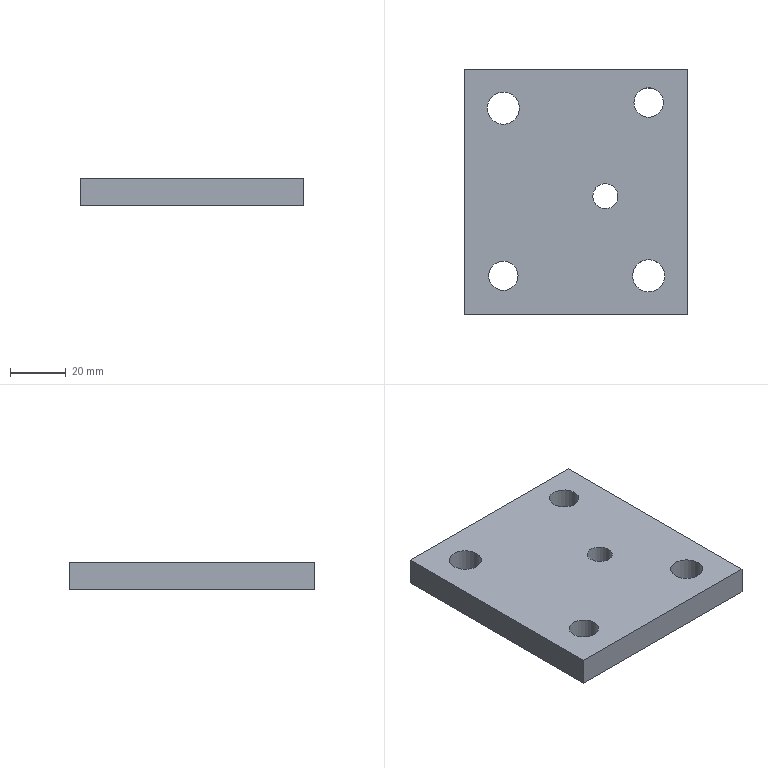Part | NX | features 6 2 | 1 solid | 11 faces | box 80 x 88 x 10 mm | volume 65955 mm3 | plane 6 | cylinder 5 | commonest cylinder face diameters 10.5 x2 11.5 x2 9 x1
STEP:
#1=CARTESIAN_POINT('',(3340.247,122.828,101.));
#2=VERTEX_POINT('',#1);
#3=CARTESIAN_POINT('',(3340.247,34.828,101.));
#4=VERTEX_POINT('',#3);
#5=CARTESIAN_POINT('',(3340.247,77.328,101.));
#6=DIRECTION('',(0.,-1.,0.));
#7=VECTOR('',#6,1000.);
#8=LINE('',#5,#7);
#9=EDGE_CURVE('',#2,#4,#8,.T.);
#10=ORIENTED_EDGE('',*,*,#9,.T.);
#11=CARTESIAN_POINT('',(3340.247,34.828,91.));
#12=VERTEX_POINT('',#11);
#13=CARTESIAN_POINT('',(3340.247,34.828,81.));
#14=DIRECTION('',(0.,0.,1.));
#15=VECTOR('',#14,1000.);
#16=LINE('',#13,#15);
#17=EDGE_CURVE('',#12,#4,#16,.T.);
#18=ORIENTED_EDGE('',*,*,#17,.F.);
#19=CARTESIAN_POINT('',(3340.247,122.828,91.));
#20=VERTEX_POINT('',#19);
#21=CARTESIAN_POINT('',(3340.247,77.328,91.));
#22=DIRECTION('',(0.,-1.,0.));
#23=VECTOR('',#22,1000.);
#24=LINE('',#21,#23);
#25=EDGE_CURVE('',#20,#12,#24,.T.);
#26=ORIENTED_EDGE('',*,*,#25,.F.);
#27=CARTESIAN_POINT('',(3340.247,122.828,81.));
#28=DIRECTION('',(0.,0.,-1.));
#29=VECTOR('',#28,1000.);
#30=LINE('',#27,#29);
#31=EDGE_CURVE('',#2,#20,#30,.T.);
#32=ORIENTED_EDGE('',*,*,#31,.F.);
#33=EDGE_LOOP('',(#10,#18,#26,#32));
#34=FACE_BOUND('',#33,.T.);
#35=CARTESIAN_POINT('',(3340.247,77.328,81.));
#36=DIRECTION('',(-1.,0.,0.));
#37=DIRECTION('',(0.,-1.,0.));
#38=AXIS2_PLACEMENT_3D('',#35,#36,#37);
#39=PLANE('',#38);
#40=ADVANCED_FACE('',(#34),#39,.F.);
#41=CARTESIAN_POINT('',(3260.247,122.828,101.));
#42=VERTEX_POINT('',#41);
#43=CARTESIAN_POINT('',(3290.247,122.828,101.));
#44=DIRECTION('',(1.,0.,0.));
#45=VECTOR('',#44,1000.);
#46=LINE('',#43,#45);
#47=EDGE_CURVE('',#42,#2,#46,.T.);
#48=ORIENTED_EDGE('',*,*,#47,.T.);
#49=ORIENTED_EDGE('',*,*,#31,.T.);
#50=CARTESIAN_POINT('',(3260.247,122.828,91.));
#51=VERTEX_POINT('',#50);
#52=CARTESIAN_POINT('',(3290.247,122.828,91.));
#53=DIRECTION('',(1.,0.,0.));
#54=VECTOR('',#53,1000.);
#55=LINE('',#52,#54);
#56=EDGE_CURVE('',#51,#20,#55,.T.);
#57=ORIENTED_EDGE('',*,*,#56,.F.);
#58=CARTESIAN_POINT('',(3260.247,122.828,81.));
#59=DIRECTION('',(0.,0.,-1.));
#60=VECTOR('',#59,1000.);
#61=LINE('',#58,#60);
#62=EDGE_CURVE('',#42,#51,#61,.T.);
#63=ORIENTED_EDGE('',*,*,#62,.F.);
#64=EDGE_LOOP('',(#48,#49,#57,#63));
#65=FACE_BOUND('',#64,.T.);
#66=CARTESIAN_POINT('',(3290.247,122.828,81.));
#67=DIRECTION('',(0.,-1.,0.));
#68=DIRECTION('',(1.,0.,0.));
#69=AXIS2_PLACEMENT_3D('',#66,#67,#68);
#70=PLANE('',#69);
#71=ADVANCED_FACE('',(#65),#70,.F.);
#72=CARTESIAN_POINT('',(3260.247,34.828,101.));
#73=VERTEX_POINT('',#72);
#74=CARTESIAN_POINT('',(3260.247,77.328,101.));
#75=DIRECTION('',(0.,1.,0.));
#76=VECTOR('',#75,1000.);
#77=LINE('',#74,#76);
#78=EDGE_CURVE('',#73,#42,#77,.T.);
#79=ORIENTED_EDGE('',*,*,#78,.T.);
#80=ORIENTED_EDGE('',*,*,#62,.T.);
#81=CARTESIAN_POINT('',(3260.247,34.828,91.));
#82=VERTEX_POINT('',#81);
#83=CARTESIAN_POINT('',(3260.247,77.328,91.));
#84=DIRECTION('',(0.,1.,0.));
#85=VECTOR('',#84,1000.);
#86=LINE('',#83,#85);
#87=EDGE_CURVE('',#82,#51,#86,.T.);
#88=ORIENTED_EDGE('',*,*,#87,.F.);
#89=CARTESIAN_POINT('',(3260.247,34.828,81.));
#90=DIRECTION('',(0.,0.,-1.));
#91=VECTOR('',#90,1000.);
#92=LINE('',#89,#91);
#93=EDGE_CURVE('',#73,#82,#92,.T.);
#94=ORIENTED_EDGE('',*,*,#93,.F.);
#95=EDGE_LOOP('',(#79,#80,#88,#94));
#96=FACE_BOUND('',#95,.T.);
#97=CARTESIAN_POINT('',(3260.247,77.328,81.));
#98=DIRECTION('',(1.,0.,0.));
#99=DIRECTION('',(0.,1.,0.));
#100=AXIS2_PLACEMENT_3D('',#97,#98,#99);
#101=PLANE('',#100);
#102=ADVANCED_FACE('',(#96),#101,.F.);
#103=CARTESIAN_POINT('',(3279.497,48.828,91.));
#104=VERTEX_POINT('',#103);
#105=CARTESIAN_POINT('',(3274.247,48.828,91.));
#106=DIRECTION('',(0.,0.,-1.));
#107=DIRECTION('',(1.,0.,0.));
#108=AXIS2_PLACEMENT_3D('',#105,#106,#107);
#109=CIRCLE('',#108,5.25);
#110=EDGE_CURVE('',#104,#104,#109,.T.);
#111=ORIENTED_EDGE('',*,*,#110,.T.);
#112=EDGE_LOOP('',(#111));
#113=FACE_BOUND('',#112,.T.);
#114=CARTESIAN_POINT('',(3268.997,48.828,101.));
#115=VERTEX_POINT('',#114);
#116=CARTESIAN_POINT('',(3274.247,48.828,101.));
#117=DIRECTION('',(0.,0.,1.));
#118=DIRECTION('',(-1.,0.,0.));
#119=AXIS2_PLACEMENT_3D('',#116,#117,#118);
#120=CIRCLE('',#119,5.25);
#121=EDGE_CURVE('',#115,#115,#120,.T.);
#122=ORIENTED_EDGE('',*,*,#121,.T.);
#123=EDGE_LOOP('',(#122));
#124=FACE_BOUND('',#123,.T.);
#125=CARTESIAN_POINT('',(3274.247,48.828,81.));
#126=DIRECTION('',(0.,0.,1.));
#127=DIRECTION('',(0.,-1.,0.));
#128=AXIS2_PLACEMENT_3D('',#125,#126,#127);
#129=CYLINDRICAL_SURFACE('',#128,5.25);
#130=ADVANCED_FACE('',(#113,#124),#129,.F.);
#131=CARTESIAN_POINT('',(3331.997,48.828,91.));
#132=VERTEX_POINT('',#131);
#133=CARTESIAN_POINT('',(3326.247,48.828,91.));
#134=DIRECTION('',(0.,0.,1.));
#135=DIRECTION('',(1.,0.,0.));
#136=AXIS2_PLACEMENT_3D('',#133,#134,#135);
#137=CIRCLE('',#136,5.75);
#138=EDGE_CURVE('',#132,#132,#137,.T.);
#139=ORIENTED_EDGE('',*,*,#138,.F.);
#140=EDGE_LOOP('',(#139));
#141=FACE_BOUND('',#140,.T.);
#142=CARTESIAN_POINT('',(3320.497,48.828,101.));
#143=VERTEX_POINT('',#142);
#144=CARTESIAN_POINT('',(3326.247,48.828,101.));
#145=DIRECTION('',(0.,0.,1.));
#146=DIRECTION('',(-1.,0.,0.));
#147=AXIS2_PLACEMENT_3D('',#144,#145,#146);
#148=CIRCLE('',#147,5.75);
#149=EDGE_CURVE('',#143,#143,#148,.T.);
#150=ORIENTED_EDGE('',*,*,#149,.T.);
#151=EDGE_LOOP('',(#150));
#152=FACE_BOUND('',#151,.T.);
#153=CARTESIAN_POINT('',(3326.247,48.828,81.));
#154=DIRECTION('',(0.,0.,1.));
#155=DIRECTION('',(0.,-1.,0.));
#156=AXIS2_PLACEMENT_3D('',#153,#154,#155);
#157=CYLINDRICAL_SURFACE('',#156,5.75);
#158=ADVANCED_FACE('',(#141,#152),#157,.F.);
#159=CARTESIAN_POINT('',(3290.247,34.828,91.));
#160=DIRECTION('',(-1.,0.,0.));
#161=VECTOR('',#160,1000.);
#162=LINE('',#159,#161);
#163=EDGE_CURVE('',#12,#82,#162,.T.);
#164=ORIENTED_EDGE('',*,*,#163,.F.);
#165=ORIENTED_EDGE('',*,*,#17,.T.);
#166=CARTESIAN_POINT('',(3290.247,34.828,101.));
#167=DIRECTION('',(-1.,0.,0.));
#168=VECTOR('',#167,1000.);
#169=LINE('',#166,#168);
#170=EDGE_CURVE('',#4,#73,#169,.T.);
#171=ORIENTED_EDGE('',*,*,#170,.T.);
#172=ORIENTED_EDGE('',*,*,#93,.T.);
#173=EDGE_LOOP('',(#164,#165,#171,#172));
#174=FACE_BOUND('',#173,.T.);
#175=CARTESIAN_POINT('',(3290.247,34.828,81.));
#176=DIRECTION('',(0.,1.,0.));
#177=DIRECTION('',(-1.,0.,0.));
#178=AXIS2_PLACEMENT_3D('',#175,#176,#177);
#179=PLANE('',#178);
#180=ADVANCED_FACE('',(#174),#179,.F.);
#181=CARTESIAN_POINT('',(3279.997,108.828,91.));
#182=VERTEX_POINT('',#181);
#183=CARTESIAN_POINT('',(3274.247,108.828,91.));
#184=DIRECTION('',(0.,0.,1.));
#185=DIRECTION('',(1.,0.,0.));
#186=AXIS2_PLACEMENT_3D('',#183,#184,#185);
#187=CIRCLE('',#186,5.75);
#188=EDGE_CURVE('',#182,#182,#187,.T.);
#189=ORIENTED_EDGE('',*,*,#188,.F.);
#190=EDGE_LOOP('',(#189));
#191=FACE_BOUND('',#190,.T.);
#192=CARTESIAN_POINT('',(3268.497,108.828,101.));
#193=VERTEX_POINT('',#192);
#194=CARTESIAN_POINT('',(3274.247,108.828,101.));
#195=DIRECTION('',(0.,0.,1.));
#196=DIRECTION('',(-1.,0.,0.));
#197=AXIS2_PLACEMENT_3D('',#194,#195,#196);
#198=CIRCLE('',#197,5.75);
#199=EDGE_CURVE('',#193,#193,#198,.T.);
#200=ORIENTED_EDGE('',*,*,#199,.T.);
#201=EDGE_LOOP('',(#200));
#202=FACE_BOUND('',#201,.T.);
#203=CARTESIAN_POINT('',(3274.247,108.828,81.));
#204=DIRECTION('',(0.,0.,1.));
#205=DIRECTION('',(0.,-1.,0.));
#206=AXIS2_PLACEMENT_3D('',#203,#204,#205);
#207=CYLINDRICAL_SURFACE('',#206,5.75);
#208=ADVANCED_FACE('',(#191,#202),#207,.F.);
#209=CARTESIAN_POINT('',(3331.497,110.828,91.));
#210=VERTEX_POINT('',#209);
#211=CARTESIAN_POINT('',(3326.247,110.828,91.));
#212=DIRECTION('',(0.,0.,-1.));
#213=DIRECTION('',(1.,0.,0.));
#214=AXIS2_PLACEMENT_3D('',#211,#212,#213);
#215=CIRCLE('',#214,5.25);
#216=EDGE_CURVE('',#210,#210,#215,.T.);
#217=ORIENTED_EDGE('',*,*,#216,.T.);
#218=EDGE_LOOP('',(#217));
#219=FACE_BOUND('',#218,.T.);
#220=CARTESIAN_POINT('',(3320.997,110.828,101.));
#221=VERTEX_POINT('',#220);
#222=CARTESIAN_POINT('',(3326.247,110.828,101.));
#223=DIRECTION('',(0.,0.,1.));
#224=DIRECTION('',(-1.,0.,0.));
#225=AXIS2_PLACEMENT_3D('',#222,#223,#224);
#226=CIRCLE('',#225,5.25);
#227=EDGE_CURVE('',#221,#221,#226,.T.);
#228=ORIENTED_EDGE('',*,*,#227,.T.);
#229=EDGE_LOOP('',(#228));
#230=FACE_BOUND('',#229,.T.);
#231=CARTESIAN_POINT('',(3326.247,110.828,81.));
#232=DIRECTION('',(0.,0.,1.));
#233=DIRECTION('',(0.,-1.,0.));
#234=AXIS2_PLACEMENT_3D('',#231,#232,#233);
#235=CYLINDRICAL_SURFACE('',#234,5.25);
#236=ADVANCED_FACE('',(#219,#230),#235,.F.);
#237=CARTESIAN_POINT('',(3315.247,77.328,91.));
#238=VERTEX_POINT('',#237);
#239=CARTESIAN_POINT('',(3310.747,77.328,91.));
#240=DIRECTION('',(0.,0.,-1.));
#241=DIRECTION('',(1.,0.,0.));
#242=AXIS2_PLACEMENT_3D('',#239,#240,#241);
#243=CIRCLE('',#242,4.5);
#244=EDGE_CURVE('',#238,#238,#243,.T.);
#245=ORIENTED_EDGE('',*,*,#244,.T.);
#246=EDGE_LOOP('',(#245));
#247=FACE_BOUND('',#246,.T.);
#248=CARTESIAN_POINT('',(3306.247,77.328,101.));
#249=VERTEX_POINT('',#248);
#250=CARTESIAN_POINT('',(3310.747,77.328,101.));
#251=DIRECTION('',(0.,0.,1.));
#252=DIRECTION('',(-1.,0.,0.));
#253=AXIS2_PLACEMENT_3D('',#250,#251,#252);
#254=CIRCLE('',#253,4.5);
#255=EDGE_CURVE('',#249,#249,#254,.T.);
#256=ORIENTED_EDGE('',*,*,#255,.T.);
#257=EDGE_LOOP('',(#256));
#258=FACE_BOUND('',#257,.T.);
#259=CARTESIAN_POINT('',(3310.747,77.328,-129.));
#260=DIRECTION('',(0.,0.,1.));
#261=DIRECTION('',(0.,-1.,0.));
#262=AXIS2_PLACEMENT_3D('',#259,#260,#261);
#263=CYLINDRICAL_SURFACE('',#262,4.5);
#264=ADVANCED_FACE('',(#247,#258),#263,.F.);
#265=ORIENTED_EDGE('',*,*,#216,.F.);
#266=EDGE_LOOP('',(#265));
#267=FACE_BOUND('',#266,.T.);
#268=ORIENTED_EDGE('',*,*,#188,.T.);
#269=EDGE_LOOP('',(#268));
#270=FACE_BOUND('',#269,.T.);
#271=ORIENTED_EDGE('',*,*,#87,.T.);
#272=ORIENTED_EDGE('',*,*,#56,.T.);
#273=ORIENTED_EDGE('',*,*,#25,.T.);
#274=ORIENTED_EDGE('',*,*,#163,.T.);
#275=EDGE_LOOP('',(#271,#272,#273,#274));
#276=FACE_BOUND('',#275,.T.);
#277=ORIENTED_EDGE('',*,*,#138,.T.);
#278=EDGE_LOOP('',(#277));
#279=FACE_BOUND('',#278,.T.);
#280=ORIENTED_EDGE('',*,*,#110,.F.);
#281=EDGE_LOOP('',(#280));
#282=FACE_BOUND('',#281,.T.);
#283=ORIENTED_EDGE('',*,*,#244,.F.);
#284=EDGE_LOOP('',(#283));
#285=FACE_BOUND('',#284,.T.);
#286=CARTESIAN_POINT('',(3290.247,77.328,91.));
#287=DIRECTION('',(0.,0.,1.));
#288=DIRECTION('',(0.,-1.,0.));
#289=AXIS2_PLACEMENT_3D('',#286,#287,#288);
#290=PLANE('',#289);
#291=ADVANCED_FACE('',(#267,#270,#276,#279,#282,#285),#290,.F.);
#292=ORIENTED_EDGE('',*,*,#121,.F.);
#293=EDGE_LOOP('',(#292));
#294=FACE_BOUND('',#293,.T.);
#295=ORIENTED_EDGE('',*,*,#149,.F.);
#296=EDGE_LOOP('',(#295));
#297=FACE_BOUND('',#296,.T.);
#298=ORIENTED_EDGE('',*,*,#170,.F.);
#299=ORIENTED_EDGE('',*,*,#9,.F.);
#300=ORIENTED_EDGE('',*,*,#47,.F.);
#301=ORIENTED_EDGE('',*,*,#78,.F.);
#302=EDGE_LOOP('',(#298,#299,#300,#301));
#303=FACE_BOUND('',#302,.T.);
#304=ORIENTED_EDGE('',*,*,#199,.F.);
#305=EDGE_LOOP('',(#304));
#306=FACE_BOUND('',#305,.T.);
#307=ORIENTED_EDGE('',*,*,#227,.F.);
#308=EDGE_LOOP('',(#307));
#309=FACE_BOUND('',#308,.T.);
#310=ORIENTED_EDGE('',*,*,#255,.F.);
#311=EDGE_LOOP('',(#310));
#312=FACE_BOUND('',#311,.T.);
#313=CARTESIAN_POINT('',(3388.056,1242.718,101.));
#314=DIRECTION('',(0.,0.,1.));
#315=DIRECTION('',(0.,1.,0.));
#316=AXIS2_PLACEMENT_3D('',#313,#314,#315);
#317=PLANE('',#316);
#318=ADVANCED_FACE('',(#294,#297,#303,#306,#309,#312),#317,.T.);
#319=CLOSED_SHELL('',(#40,#71,#102,#130,#158,#180,#208,#236,#264,#291,#318));
#320=MANIFOLD_SOLID_BREP('',#319);
#321=(LENGTH_UNIT()NAMED_UNIT(*)SI_UNIT(.MILLI.,.METRE.));
#322=UNCERTAINTY_MEASURE_WITH_UNIT(LENGTH_MEASURE(0.00001),#321,'','');
#323=(NAMED_UNIT(*)PLANE_ANGLE_UNIT()SI_UNIT($,.RADIAN.));
#324=(NAMED_UNIT(*)SI_UNIT($,.STERADIAN.)SOLID_ANGLE_UNIT());
#325=(GEOMETRIC_REPRESENTATION_CONTEXT(3)GLOBAL_UNCERTAINTY_ASSIGNED_CONTEXT((#322))GLOBAL_UNIT_ASSIGNED_CONTEXT((#321,#323,#324))REPRESENTATION_CONTEXT('',''));
#326=ADVANCED_BREP_SHAPE_REPRESENTATION('',(#320),#325);